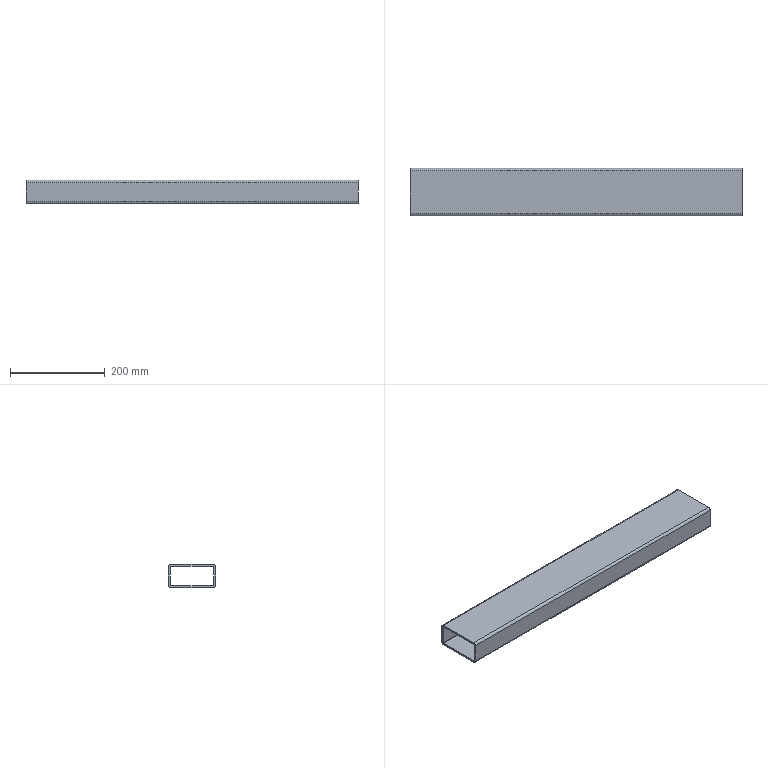Part | SolidWorks | features BaseBody 1 | 1 solid | 18 faces | box 700 x 100 x 50 mm | volume 780779 mm3 | plane 10 | cylinder 8 | commonest cylinder face diameters 2 x4 10 x4
STEP:
#1=CARTESIAN_POINT('',(-350.,45.,-25.));
#2=VERTEX_POINT('',#1);
#3=CARTESIAN_POINT('',(-350.,50.,-20.));
#4=VERTEX_POINT('',#3);
#5=CARTESIAN_POINT('',(-350.,45.,-20.));
#6=DIRECTION('',(1.,0.,0.));
#7=DIRECTION('',(0.,0.,-1.));
#8=AXIS2_PLACEMENT_3D('',#5,#6,#7);
#9=CIRCLE('',#8,5.);
#10=EDGE_CURVE('',#2,#4,#9,.T.);
#11=ORIENTED_EDGE('',*,*,#10,.T.);
#12=CARTESIAN_POINT('',(350.,50.,-20.));
#13=VERTEX_POINT('',#12);
#14=CARTESIAN_POINT('',(350.,50.,-20.));
#15=DIRECTION('',(-1.,0.,0.));
#16=VECTOR('',#15,1000.);
#17=LINE('',#14,#16);
#18=EDGE_CURVE('',#13,#4,#17,.T.);
#19=ORIENTED_EDGE('',*,*,#18,.F.);
#20=CARTESIAN_POINT('',(350.,45.,-25.));
#21=VERTEX_POINT('',#20);
#22=CARTESIAN_POINT('',(350.,45.,-20.));
#23=DIRECTION('',(1.,0.,0.));
#24=DIRECTION('',(0.,0.,-1.));
#25=AXIS2_PLACEMENT_3D('',#22,#23,#24);
#26=CIRCLE('',#25,5.);
#27=EDGE_CURVE('',#21,#13,#26,.T.);
#28=ORIENTED_EDGE('',*,*,#27,.F.);
#29=CARTESIAN_POINT('',(350.,45.,-25.));
#30=DIRECTION('',(-1.,0.,0.));
#31=VECTOR('',#30,1000.);
#32=LINE('',#29,#31);
#33=EDGE_CURVE('',#21,#2,#32,.T.);
#34=ORIENTED_EDGE('',*,*,#33,.T.);
#35=EDGE_LOOP('',(#11,#19,#28,#34));
#36=FACE_OUTER_BOUND('',#35,.T.);
#37=CARTESIAN_POINT('',(350.,45.,-20.));
#38=DIRECTION('',(-1.,0.,0.));
#39=DIRECTION('',(0.,0.,1.));
#40=AXIS2_PLACEMENT_3D('',#37,#38,#39);
#41=CYLINDRICAL_SURFACE('',#40,5.);
#42=ADVANCED_FACE('',(#36),#41,.T.);
#43=CARTESIAN_POINT('',(-350.,50.,20.));
#44=VERTEX_POINT('',#43);
#45=CARTESIAN_POINT('',(-350.,50.,-20.));
#46=DIRECTION('',(0.,0.,1.));
#47=VECTOR('',#46,1000.);
#48=LINE('',#45,#47);
#49=EDGE_CURVE('',#4,#44,#48,.T.);
#50=ORIENTED_EDGE('',*,*,#49,.T.);
#51=CARTESIAN_POINT('',(350.,50.,20.));
#52=VERTEX_POINT('',#51);
#53=CARTESIAN_POINT('',(350.,50.,20.));
#54=DIRECTION('',(-1.,0.,0.));
#55=VECTOR('',#54,1000.);
#56=LINE('',#53,#55);
#57=EDGE_CURVE('',#52,#44,#56,.T.);
#58=ORIENTED_EDGE('',*,*,#57,.F.);
#59=CARTESIAN_POINT('',(350.,50.,-20.));
#60=DIRECTION('',(0.,0.,1.));
#61=VECTOR('',#60,1000.);
#62=LINE('',#59,#61);
#63=EDGE_CURVE('',#13,#52,#62,.T.);
#64=ORIENTED_EDGE('',*,*,#63,.F.);
#65=ORIENTED_EDGE('',*,*,#18,.T.);
#66=EDGE_LOOP('',(#50,#58,#64,#65));
#67=FACE_OUTER_BOUND('',#66,.T.);
#68=CARTESIAN_POINT('',(350.,50.,-20.));
#69=DIRECTION('',(0.,-1.,0.));
#70=DIRECTION('',(0.,0.,-1.));
#71=AXIS2_PLACEMENT_3D('',#68,#69,#70);
#72=PLANE('',#71);
#73=ADVANCED_FACE('',(#67),#72,.F.);
#74=CARTESIAN_POINT('',(-350.,45.,25.));
#75=VERTEX_POINT('',#74);
#76=CARTESIAN_POINT('',(-350.,45.,20.));
#77=DIRECTION('',(1.,0.,0.));
#78=DIRECTION('',(0.,0.,-1.));
#79=AXIS2_PLACEMENT_3D('',#76,#77,#78);
#80=CIRCLE('',#79,5.);
#81=EDGE_CURVE('',#44,#75,#80,.T.);
#82=ORIENTED_EDGE('',*,*,#81,.T.);
#83=CARTESIAN_POINT('',(350.,45.,25.));
#84=VERTEX_POINT('',#83);
#85=CARTESIAN_POINT('',(350.,45.,25.));
#86=DIRECTION('',(-1.,0.,0.));
#87=VECTOR('',#86,1000.);
#88=LINE('',#85,#87);
#89=EDGE_CURVE('',#84,#75,#88,.T.);
#90=ORIENTED_EDGE('',*,*,#89,.F.);
#91=CARTESIAN_POINT('',(350.,45.,20.));
#92=DIRECTION('',(1.,0.,0.));
#93=DIRECTION('',(0.,0.,-1.));
#94=AXIS2_PLACEMENT_3D('',#91,#92,#93);
#95=CIRCLE('',#94,5.);
#96=EDGE_CURVE('',#52,#84,#95,.T.);
#97=ORIENTED_EDGE('',*,*,#96,.F.);
#98=ORIENTED_EDGE('',*,*,#57,.T.);
#99=EDGE_LOOP('',(#82,#90,#97,#98));
#100=FACE_OUTER_BOUND('',#99,.T.);
#101=CARTESIAN_POINT('',(350.,45.,20.));
#102=DIRECTION('',(-1.,0.,0.));
#103=DIRECTION('',(0.,0.,1.));
#104=AXIS2_PLACEMENT_3D('',#101,#102,#103);
#105=CYLINDRICAL_SURFACE('',#104,5.);
#106=ADVANCED_FACE('',(#100),#105,.T.);
#107=CARTESIAN_POINT('',(-350.,-45.,25.));
#108=VERTEX_POINT('',#107);
#109=CARTESIAN_POINT('',(-350.,-45.,25.));
#110=DIRECTION('',(0.,-1.,0.));
#111=VECTOR('',#110,1000.);
#112=LINE('',#109,#111);
#113=EDGE_CURVE('',#75,#108,#112,.T.);
#114=ORIENTED_EDGE('',*,*,#113,.T.);
#115=CARTESIAN_POINT('',(350.,-45.,25.));
#116=VERTEX_POINT('',#115);
#117=CARTESIAN_POINT('',(350.,-45.,25.));
#118=DIRECTION('',(-1.,0.,0.));
#119=VECTOR('',#118,1000.);
#120=LINE('',#117,#119);
#121=EDGE_CURVE('',#116,#108,#120,.T.);
#122=ORIENTED_EDGE('',*,*,#121,.F.);
#123=CARTESIAN_POINT('',(350.,-45.,25.));
#124=DIRECTION('',(0.,-1.,0.));
#125=VECTOR('',#124,1000.);
#126=LINE('',#123,#125);
#127=EDGE_CURVE('',#84,#116,#126,.T.);
#128=ORIENTED_EDGE('',*,*,#127,.F.);
#129=ORIENTED_EDGE('',*,*,#89,.T.);
#130=EDGE_LOOP('',(#114,#122,#128,#129));
#131=FACE_OUTER_BOUND('',#130,.T.);
#132=CARTESIAN_POINT('',(350.,-45.,25.));
#133=DIRECTION('',(0.,0.,-1.));
#134=DIRECTION('',(0.,1.,0.));
#135=AXIS2_PLACEMENT_3D('',#132,#133,#134);
#136=PLANE('',#135);
#137=ADVANCED_FACE('',(#131),#136,.F.);
#138=CARTESIAN_POINT('',(-350.,-50.,20.));
#139=VERTEX_POINT('',#138);
#140=CARTESIAN_POINT('',(-350.,-45.,20.));
#141=DIRECTION('',(1.,0.,0.));
#142=DIRECTION('',(0.,0.,-1.));
#143=AXIS2_PLACEMENT_3D('',#140,#141,#142);
#144=CIRCLE('',#143,5.);
#145=EDGE_CURVE('',#108,#139,#144,.T.);
#146=ORIENTED_EDGE('',*,*,#145,.T.);
#147=CARTESIAN_POINT('',(350.,-50.,20.));
#148=VERTEX_POINT('',#147);
#149=CARTESIAN_POINT('',(350.,-50.,20.));
#150=DIRECTION('',(-1.,0.,0.));
#151=VECTOR('',#150,1000.);
#152=LINE('',#149,#151);
#153=EDGE_CURVE('',#148,#139,#152,.T.);
#154=ORIENTED_EDGE('',*,*,#153,.F.);
#155=CARTESIAN_POINT('',(350.,-45.,20.));
#156=DIRECTION('',(1.,0.,0.));
#157=DIRECTION('',(0.,0.,-1.));
#158=AXIS2_PLACEMENT_3D('',#155,#156,#157);
#159=CIRCLE('',#158,5.);
#160=EDGE_CURVE('',#116,#148,#159,.T.);
#161=ORIENTED_EDGE('',*,*,#160,.F.);
#162=ORIENTED_EDGE('',*,*,#121,.T.);
#163=EDGE_LOOP('',(#146,#154,#161,#162));
#164=FACE_OUTER_BOUND('',#163,.T.);
#165=CARTESIAN_POINT('',(350.,-45.,20.));
#166=DIRECTION('',(-1.,0.,0.));
#167=DIRECTION('',(0.,0.,1.));
#168=AXIS2_PLACEMENT_3D('',#165,#166,#167);
#169=CYLINDRICAL_SURFACE('',#168,5.);
#170=ADVANCED_FACE('',(#164),#169,.T.);
#171=CARTESIAN_POINT('',(-350.,-50.,-20.));
#172=VERTEX_POINT('',#171);
#173=CARTESIAN_POINT('',(-350.,-50.,20.));
#174=DIRECTION('',(0.,0.,-1.));
#175=VECTOR('',#174,1000.);
#176=LINE('',#173,#175);
#177=EDGE_CURVE('',#139,#172,#176,.T.);
#178=ORIENTED_EDGE('',*,*,#177,.T.);
#179=CARTESIAN_POINT('',(350.,-50.,-20.));
#180=VERTEX_POINT('',#179);
#181=CARTESIAN_POINT('',(350.,-50.,-20.));
#182=DIRECTION('',(-1.,0.,0.));
#183=VECTOR('',#182,1000.);
#184=LINE('',#181,#183);
#185=EDGE_CURVE('',#180,#172,#184,.T.);
#186=ORIENTED_EDGE('',*,*,#185,.F.);
#187=CARTESIAN_POINT('',(350.,-50.,20.));
#188=DIRECTION('',(0.,0.,-1.));
#189=VECTOR('',#188,1000.);
#190=LINE('',#187,#189);
#191=EDGE_CURVE('',#148,#180,#190,.T.);
#192=ORIENTED_EDGE('',*,*,#191,.F.);
#193=ORIENTED_EDGE('',*,*,#153,.T.);
#194=EDGE_LOOP('',(#178,#186,#192,#193));
#195=FACE_OUTER_BOUND('',#194,.T.);
#196=CARTESIAN_POINT('',(350.,-50.,20.));
#197=DIRECTION('',(0.,1.,0.));
#198=DIRECTION('',(0.,0.,1.));
#199=AXIS2_PLACEMENT_3D('',#196,#197,#198);
#200=PLANE('',#199);
#201=ADVANCED_FACE('',(#195),#200,.F.);
#202=CARTESIAN_POINT('',(-350.,-45.,-25.));
#203=VERTEX_POINT('',#202);
#204=CARTESIAN_POINT('',(-350.,-45.,-20.));
#205=DIRECTION('',(1.,0.,0.));
#206=DIRECTION('',(0.,0.,-1.));
#207=AXIS2_PLACEMENT_3D('',#204,#205,#206);
#208=CIRCLE('',#207,5.);
#209=EDGE_CURVE('',#172,#203,#208,.T.);
#210=ORIENTED_EDGE('',*,*,#209,.T.);
#211=CARTESIAN_POINT('',(350.,-45.,-25.));
#212=VERTEX_POINT('',#211);
#213=CARTESIAN_POINT('',(350.,-45.,-25.));
#214=DIRECTION('',(-1.,0.,0.));
#215=VECTOR('',#214,1000.);
#216=LINE('',#213,#215);
#217=EDGE_CURVE('',#212,#203,#216,.T.);
#218=ORIENTED_EDGE('',*,*,#217,.F.);
#219=CARTESIAN_POINT('',(350.,-45.,-20.));
#220=DIRECTION('',(1.,0.,0.));
#221=DIRECTION('',(0.,0.,-1.));
#222=AXIS2_PLACEMENT_3D('',#219,#220,#221);
#223=CIRCLE('',#222,5.);
#224=EDGE_CURVE('',#180,#212,#223,.T.);
#225=ORIENTED_EDGE('',*,*,#224,.F.);
#226=ORIENTED_EDGE('',*,*,#185,.T.);
#227=EDGE_LOOP('',(#210,#218,#225,#226));
#228=FACE_OUTER_BOUND('',#227,.T.);
#229=CARTESIAN_POINT('',(350.,-45.,-20.));
#230=DIRECTION('',(-1.,0.,0.));
#231=DIRECTION('',(0.,0.,1.));
#232=AXIS2_PLACEMENT_3D('',#229,#230,#231);
#233=CYLINDRICAL_SURFACE('',#232,5.);
#234=ADVANCED_FACE('',(#228),#233,.T.);
#235=CARTESIAN_POINT('',(-350.,46.,20.));
#236=VERTEX_POINT('',#235);
#237=CARTESIAN_POINT('',(-350.,45.,21.));
#238=VERTEX_POINT('',#237);
#239=CARTESIAN_POINT('',(-350.,45.,20.));
#240=DIRECTION('',(1.,0.,0.));
#241=DIRECTION('',(0.,0.,-1.));
#242=AXIS2_PLACEMENT_3D('',#239,#240,#241);
#243=CIRCLE('',#242,1.);
#244=EDGE_CURVE('',#236,#238,#243,.T.);
#245=ORIENTED_EDGE('',*,*,#244,.F.);
#246=CARTESIAN_POINT('',(350.,46.,20.));
#247=VERTEX_POINT('',#246);
#248=CARTESIAN_POINT('',(350.,46.,20.));
#249=DIRECTION('',(-1.,0.,0.));
#250=VECTOR('',#249,1000.);
#251=LINE('',#248,#250);
#252=EDGE_CURVE('',#247,#236,#251,.T.);
#253=ORIENTED_EDGE('',*,*,#252,.F.);
#254=CARTESIAN_POINT('',(350.,45.,21.));
#255=VERTEX_POINT('',#254);
#256=CARTESIAN_POINT('',(350.,45.,20.));
#257=DIRECTION('',(1.,0.,0.));
#258=DIRECTION('',(0.,0.,-1.));
#259=AXIS2_PLACEMENT_3D('',#256,#257,#258);
#260=CIRCLE('',#259,1.);
#261=EDGE_CURVE('',#247,#255,#260,.T.);
#262=ORIENTED_EDGE('',*,*,#261,.T.);
#263=CARTESIAN_POINT('',(350.,45.,21.));
#264=DIRECTION('',(-1.,0.,0.));
#265=VECTOR('',#264,1000.);
#266=LINE('',#263,#265);
#267=EDGE_CURVE('',#255,#238,#266,.T.);
#268=ORIENTED_EDGE('',*,*,#267,.T.);
#269=EDGE_LOOP('',(#245,#253,#262,#268));
#270=FACE_OUTER_BOUND('',#269,.T.);
#271=CARTESIAN_POINT('',(350.,45.,20.));
#272=DIRECTION('',(-1.,0.,0.));
#273=DIRECTION('',(0.,0.,1.));
#274=AXIS2_PLACEMENT_3D('',#271,#272,#273);
#275=CYLINDRICAL_SURFACE('',#274,1.);
#276=ADVANCED_FACE('',(#270),#275,.F.);
#277=CARTESIAN_POINT('',(-350.,46.,-20.));
#278=VERTEX_POINT('',#277);
#279=CARTESIAN_POINT('',(-350.,46.,-20.));
#280=DIRECTION('',(0.,0.,1.));
#281=VECTOR('',#280,1000.);
#282=LINE('',#279,#281);
#283=EDGE_CURVE('',#278,#236,#282,.T.);
#284=ORIENTED_EDGE('',*,*,#283,.F.);
#285=CARTESIAN_POINT('',(350.,46.,-20.));
#286=VERTEX_POINT('',#285);
#287=CARTESIAN_POINT('',(350.,46.,-20.));
#288=DIRECTION('',(-1.,0.,0.));
#289=VECTOR('',#288,1000.);
#290=LINE('',#287,#289);
#291=EDGE_CURVE('',#286,#278,#290,.T.);
#292=ORIENTED_EDGE('',*,*,#291,.F.);
#293=CARTESIAN_POINT('',(350.,46.,-20.));
#294=DIRECTION('',(0.,0.,1.));
#295=VECTOR('',#294,1000.);
#296=LINE('',#293,#295);
#297=EDGE_CURVE('',#286,#247,#296,.T.);
#298=ORIENTED_EDGE('',*,*,#297,.T.);
#299=ORIENTED_EDGE('',*,*,#252,.T.);
#300=EDGE_LOOP('',(#284,#292,#298,#299));
#301=FACE_OUTER_BOUND('',#300,.T.);
#302=CARTESIAN_POINT('',(350.,46.,-20.));
#303=DIRECTION('',(0.,-1.,0.));
#304=DIRECTION('',(0.,0.,-1.));
#305=AXIS2_PLACEMENT_3D('',#302,#303,#304);
#306=PLANE('',#305);
#307=ADVANCED_FACE('',(#301),#306,.T.);
#308=CARTESIAN_POINT('',(-350.,45.,-21.));
#309=VERTEX_POINT('',#308);
#310=CARTESIAN_POINT('',(-350.,45.,-20.));
#311=DIRECTION('',(1.,0.,0.));
#312=DIRECTION('',(0.,0.,-1.));
#313=AXIS2_PLACEMENT_3D('',#310,#311,#312);
#314=CIRCLE('',#313,1.);
#315=EDGE_CURVE('',#309,#278,#314,.T.);
#316=ORIENTED_EDGE('',*,*,#315,.F.);
#317=CARTESIAN_POINT('',(350.,45.,-21.));
#318=VERTEX_POINT('',#317);
#319=CARTESIAN_POINT('',(350.,45.,-21.));
#320=DIRECTION('',(-1.,0.,0.));
#321=VECTOR('',#320,1000.);
#322=LINE('',#319,#321);
#323=EDGE_CURVE('',#318,#309,#322,.T.);
#324=ORIENTED_EDGE('',*,*,#323,.F.);
#325=CARTESIAN_POINT('',(350.,45.,-20.));
#326=DIRECTION('',(1.,0.,0.));
#327=DIRECTION('',(0.,0.,-1.));
#328=AXIS2_PLACEMENT_3D('',#325,#326,#327);
#329=CIRCLE('',#328,1.);
#330=EDGE_CURVE('',#318,#286,#329,.T.);
#331=ORIENTED_EDGE('',*,*,#330,.T.);
#332=ORIENTED_EDGE('',*,*,#291,.T.);
#333=EDGE_LOOP('',(#316,#324,#331,#332));
#334=FACE_OUTER_BOUND('',#333,.T.);
#335=CARTESIAN_POINT('',(350.,45.,-20.));
#336=DIRECTION('',(-1.,0.,0.));
#337=DIRECTION('',(0.,0.,1.));
#338=AXIS2_PLACEMENT_3D('',#335,#336,#337);
#339=CYLINDRICAL_SURFACE('',#338,1.);
#340=ADVANCED_FACE('',(#334),#339,.F.);
#341=CARTESIAN_POINT('',(-350.,-45.,-21.));
#342=VERTEX_POINT('',#341);
#343=CARTESIAN_POINT('',(-350.,45.,-21.));
#344=DIRECTION('',(0.,1.,0.));
#345=VECTOR('',#344,1000.);
#346=LINE('',#343,#345);
#347=EDGE_CURVE('',#342,#309,#346,.T.);
#348=ORIENTED_EDGE('',*,*,#347,.F.);
#349=CARTESIAN_POINT('',(350.,-45.,-21.));
#350=VERTEX_POINT('',#349);
#351=CARTESIAN_POINT('',(350.,-45.,-21.));
#352=DIRECTION('',(-1.,0.,0.));
#353=VECTOR('',#352,1000.);
#354=LINE('',#351,#353);
#355=EDGE_CURVE('',#350,#342,#354,.T.);
#356=ORIENTED_EDGE('',*,*,#355,.F.);
#357=CARTESIAN_POINT('',(350.,45.,-21.));
#358=DIRECTION('',(0.,1.,0.));
#359=VECTOR('',#358,1000.);
#360=LINE('',#357,#359);
#361=EDGE_CURVE('',#350,#318,#360,.T.);
#362=ORIENTED_EDGE('',*,*,#361,.T.);
#363=ORIENTED_EDGE('',*,*,#323,.T.);
#364=EDGE_LOOP('',(#348,#356,#362,#363));
#365=FACE_OUTER_BOUND('',#364,.T.);
#366=CARTESIAN_POINT('',(350.,45.,-21.));
#367=DIRECTION('',(0.,0.,1.));
#368=DIRECTION('',(1.,0.,0.));
#369=AXIS2_PLACEMENT_3D('',#366,#367,#368);
#370=PLANE('',#369);
#371=ADVANCED_FACE('',(#365),#370,.T.);
#372=CARTESIAN_POINT('',(-350.,-46.,-20.));
#373=VERTEX_POINT('',#372);
#374=CARTESIAN_POINT('',(-350.,-45.,-20.));
#375=DIRECTION('',(1.,0.,0.));
#376=DIRECTION('',(0.,0.,-1.));
#377=AXIS2_PLACEMENT_3D('',#374,#375,#376);
#378=CIRCLE('',#377,1.);
#379=EDGE_CURVE('',#373,#342,#378,.T.);
#380=ORIENTED_EDGE('',*,*,#379,.F.);
#381=CARTESIAN_POINT('',(350.,-46.,-20.));
#382=VERTEX_POINT('',#381);
#383=CARTESIAN_POINT('',(350.,-46.,-20.));
#384=DIRECTION('',(-1.,0.,0.));
#385=VECTOR('',#384,1000.);
#386=LINE('',#383,#385);
#387=EDGE_CURVE('',#382,#373,#386,.T.);
#388=ORIENTED_EDGE('',*,*,#387,.F.);
#389=CARTESIAN_POINT('',(350.,-45.,-20.));
#390=DIRECTION('',(1.,0.,0.));
#391=DIRECTION('',(0.,0.,-1.));
#392=AXIS2_PLACEMENT_3D('',#389,#390,#391);
#393=CIRCLE('',#392,1.);
#394=EDGE_CURVE('',#382,#350,#393,.T.);
#395=ORIENTED_EDGE('',*,*,#394,.T.);
#396=ORIENTED_EDGE('',*,*,#355,.T.);
#397=EDGE_LOOP('',(#380,#388,#395,#396));
#398=FACE_OUTER_BOUND('',#397,.T.);
#399=CARTESIAN_POINT('',(350.,-45.,-20.));
#400=DIRECTION('',(-1.,0.,0.));
#401=DIRECTION('',(0.,0.,1.));
#402=AXIS2_PLACEMENT_3D('',#399,#400,#401);
#403=CYLINDRICAL_SURFACE('',#402,1.);
#404=ADVANCED_FACE('',(#398),#403,.F.);
#405=CARTESIAN_POINT('',(-350.,-46.,20.));
#406=VERTEX_POINT('',#405);
#407=CARTESIAN_POINT('',(-350.,-46.,20.));
#408=DIRECTION('',(0.,0.,-1.));
#409=VECTOR('',#408,1000.);
#410=LINE('',#407,#409);
#411=EDGE_CURVE('',#406,#373,#410,.T.);
#412=ORIENTED_EDGE('',*,*,#411,.F.);
#413=CARTESIAN_POINT('',(350.,-46.,20.));
#414=VERTEX_POINT('',#413);
#415=CARTESIAN_POINT('',(350.,-46.,20.));
#416=DIRECTION('',(-1.,0.,0.));
#417=VECTOR('',#416,1000.);
#418=LINE('',#415,#417);
#419=EDGE_CURVE('',#414,#406,#418,.T.);
#420=ORIENTED_EDGE('',*,*,#419,.F.);
#421=CARTESIAN_POINT('',(350.,-46.,20.));
#422=DIRECTION('',(0.,0.,-1.));
#423=VECTOR('',#422,1000.);
#424=LINE('',#421,#423);
#425=EDGE_CURVE('',#414,#382,#424,.T.);
#426=ORIENTED_EDGE('',*,*,#425,.T.);
#427=ORIENTED_EDGE('',*,*,#387,.T.);
#428=EDGE_LOOP('',(#412,#420,#426,#427));
#429=FACE_OUTER_BOUND('',#428,.T.);
#430=CARTESIAN_POINT('',(350.,-46.,20.));
#431=DIRECTION('',(0.,1.,0.));
#432=DIRECTION('',(0.,0.,1.));
#433=AXIS2_PLACEMENT_3D('',#430,#431,#432);
#434=PLANE('',#433);
#435=ADVANCED_FACE('',(#429),#434,.T.);
#436=CARTESIAN_POINT('',(-350.,-45.,21.));
#437=VERTEX_POINT('',#436);
#438=CARTESIAN_POINT('',(-350.,-45.,20.));
#439=DIRECTION('',(1.,0.,0.));
#440=DIRECTION('',(0.,0.,-1.));
#441=AXIS2_PLACEMENT_3D('',#438,#439,#440);
#442=CIRCLE('',#441,1.);
#443=EDGE_CURVE('',#437,#406,#442,.T.);
#444=ORIENTED_EDGE('',*,*,#443,.F.);
#445=CARTESIAN_POINT('',(350.,-45.,21.));
#446=VERTEX_POINT('',#445);
#447=CARTESIAN_POINT('',(350.,-45.,21.));
#448=DIRECTION('',(-1.,0.,0.));
#449=VECTOR('',#448,1000.);
#450=LINE('',#447,#449);
#451=EDGE_CURVE('',#446,#437,#450,.T.);
#452=ORIENTED_EDGE('',*,*,#451,.F.);
#453=CARTESIAN_POINT('',(350.,-45.,20.));
#454=DIRECTION('',(1.,0.,0.));
#455=DIRECTION('',(0.,0.,-1.));
#456=AXIS2_PLACEMENT_3D('',#453,#454,#455);
#457=CIRCLE('',#456,1.);
#458=EDGE_CURVE('',#446,#414,#457,.T.);
#459=ORIENTED_EDGE('',*,*,#458,.T.);
#460=ORIENTED_EDGE('',*,*,#419,.T.);
#461=EDGE_LOOP('',(#444,#452,#459,#460));
#462=FACE_OUTER_BOUND('',#461,.T.);
#463=CARTESIAN_POINT('',(350.,-45.,20.));
#464=DIRECTION('',(-1.,0.,0.));
#465=DIRECTION('',(0.,0.,1.));
#466=AXIS2_PLACEMENT_3D('',#463,#464,#465);
#467=CYLINDRICAL_SURFACE('',#466,1.);
#468=ADVANCED_FACE('',(#462),#467,.F.);
#469=CARTESIAN_POINT('',(-350.,-45.,21.));
#470=DIRECTION('',(0.,-1.,0.));
#471=VECTOR('',#470,1000.);
#472=LINE('',#469,#471);
#473=EDGE_CURVE('',#238,#437,#472,.T.);
#474=ORIENTED_EDGE('',*,*,#473,.F.);
#475=ORIENTED_EDGE('',*,*,#267,.F.);
#476=CARTESIAN_POINT('',(350.,-45.,21.));
#477=DIRECTION('',(0.,-1.,0.));
#478=VECTOR('',#477,1000.);
#479=LINE('',#476,#478);
#480=EDGE_CURVE('',#255,#446,#479,.T.);
#481=ORIENTED_EDGE('',*,*,#480,.T.);
#482=ORIENTED_EDGE('',*,*,#451,.T.);
#483=EDGE_LOOP('',(#474,#475,#481,#482));
#484=FACE_OUTER_BOUND('',#483,.T.);
#485=CARTESIAN_POINT('',(350.,-45.,21.));
#486=DIRECTION('',(0.,0.,-1.));
#487=DIRECTION('',(0.,1.,0.));
#488=AXIS2_PLACEMENT_3D('',#485,#486,#487);
#489=PLANE('',#488);
#490=ADVANCED_FACE('',(#484),#489,.T.);
#491=CARTESIAN_POINT('',(-350.,45.,-25.));
#492=DIRECTION('',(0.,1.,0.));
#493=VECTOR('',#492,1000.);
#494=LINE('',#491,#493);
#495=EDGE_CURVE('',#203,#2,#494,.T.);
#496=ORIENTED_EDGE('',*,*,#495,.T.);
#497=ORIENTED_EDGE('',*,*,#33,.F.);
#498=CARTESIAN_POINT('',(350.,45.,-25.));
#499=DIRECTION('',(0.,1.,0.));
#500=VECTOR('',#499,1000.);
#501=LINE('',#498,#500);
#502=EDGE_CURVE('',#212,#21,#501,.T.);
#503=ORIENTED_EDGE('',*,*,#502,.F.);
#504=ORIENTED_EDGE('',*,*,#217,.T.);
#505=EDGE_LOOP('',(#496,#497,#503,#504));
#506=FACE_OUTER_BOUND('',#505,.T.);
#507=CARTESIAN_POINT('',(350.,45.,-25.));
#508=DIRECTION('',(0.,0.,1.));
#509=DIRECTION('',(1.,0.,0.));
#510=AXIS2_PLACEMENT_3D('',#507,#508,#509);
#511=PLANE('',#510);
#512=ADVANCED_FACE('',(#506),#511,.F.);
#513=ORIENTED_EDGE('',*,*,#261,.F.);
#514=ORIENTED_EDGE('',*,*,#297,.F.);
#515=ORIENTED_EDGE('',*,*,#330,.F.);
#516=ORIENTED_EDGE('',*,*,#361,.F.);
#517=ORIENTED_EDGE('',*,*,#394,.F.);
#518=ORIENTED_EDGE('',*,*,#425,.F.);
#519=ORIENTED_EDGE('',*,*,#458,.F.);
#520=ORIENTED_EDGE('',*,*,#480,.F.);
#521=EDGE_LOOP('',(#513,#514,#515,#516,#517,#518,#519,#520));
#522=FACE_BOUND('',#521,.T.);
#523=ORIENTED_EDGE('',*,*,#27,.T.);
#524=ORIENTED_EDGE('',*,*,#63,.T.);
#525=ORIENTED_EDGE('',*,*,#96,.T.);
#526=ORIENTED_EDGE('',*,*,#127,.T.);
#527=ORIENTED_EDGE('',*,*,#160,.T.);
#528=ORIENTED_EDGE('',*,*,#191,.T.);
#529=ORIENTED_EDGE('',*,*,#224,.T.);
#530=ORIENTED_EDGE('',*,*,#502,.T.);
#531=EDGE_LOOP('',(#523,#524,#525,#526,#527,#528,#529,#530));
#532=FACE_OUTER_BOUND('',#531,.T.);
#533=CARTESIAN_POINT('',(350.,45.,-20.));
#534=DIRECTION('',(1.,0.,0.));
#535=DIRECTION('',(0.,0.,-1.));
#536=AXIS2_PLACEMENT_3D('',#533,#534,#535);
#537=PLANE('',#536);
#538=ADVANCED_FACE('',(#522,#532),#537,.T.);
#539=ORIENTED_EDGE('',*,*,#244,.T.);
#540=ORIENTED_EDGE('',*,*,#473,.T.);
#541=ORIENTED_EDGE('',*,*,#443,.T.);
#542=ORIENTED_EDGE('',*,*,#411,.T.);
#543=ORIENTED_EDGE('',*,*,#379,.T.);
#544=ORIENTED_EDGE('',*,*,#347,.T.);
#545=ORIENTED_EDGE('',*,*,#315,.T.);
#546=ORIENTED_EDGE('',*,*,#283,.T.);
#547=EDGE_LOOP('',(#539,#540,#541,#542,#543,#544,#545,#546));
#548=FACE_BOUND('',#547,.T.);
#549=ORIENTED_EDGE('',*,*,#10,.F.);
#550=ORIENTED_EDGE('',*,*,#495,.F.);
#551=ORIENTED_EDGE('',*,*,#209,.F.);
#552=ORIENTED_EDGE('',*,*,#177,.F.);
#553=ORIENTED_EDGE('',*,*,#145,.F.);
#554=ORIENTED_EDGE('',*,*,#113,.F.);
#555=ORIENTED_EDGE('',*,*,#81,.F.);
#556=ORIENTED_EDGE('',*,*,#49,.F.);
#557=EDGE_LOOP('',(#549,#550,#551,#552,#553,#554,#555,#556));
#558=FACE_OUTER_BOUND('',#557,.T.);
#559=CARTESIAN_POINT('',(-350.,45.,-20.));
#560=DIRECTION('',(1.,0.,0.));
#561=DIRECTION('',(0.,0.,-1.));
#562=AXIS2_PLACEMENT_3D('',#559,#560,#561);
#563=PLANE('',#562);
#564=ADVANCED_FACE('',(#548,#558),#563,.F.);
#565=CLOSED_SHELL('',(#42,#73,#106,#137,#170,#201,#234,#276,#307,#340,#371,#404,#435,#468,#490,#512,#538,#564));
#566=MANIFOLD_SOLID_BREP('',#565);
#567=CARTESIAN_POINT('',(0.,0.,0.));
#568=DIRECTION('',(0.,0.,1.));
#569=DIRECTION('',(1.,0.,0.));
#570=AXIS2_PLACEMENT_3D('',#567,#568,#569);
#571=(LENGTH_UNIT()NAMED_UNIT(*)SI_UNIT(.MILLI.,.METRE.));
#572=UNCERTAINTY_MEASURE_WITH_UNIT(LENGTH_MEASURE(0.00001),#571,'','');
#573=(NAMED_UNIT(*)PLANE_ANGLE_UNIT()SI_UNIT($,.RADIAN.));
#574=(NAMED_UNIT(*)SI_UNIT($,.STERADIAN.)SOLID_ANGLE_UNIT());
#575=(GEOMETRIC_REPRESENTATION_CONTEXT(3)GLOBAL_UNCERTAINTY_ASSIGNED_CONTEXT((#572))GLOBAL_UNIT_ASSIGNED_CONTEXT((#571,#573,#574))REPRESENTATION_CONTEXT('',''));
#576=ADVANCED_BREP_SHAPE_REPRESENTATION('',(#566,#570),#575);